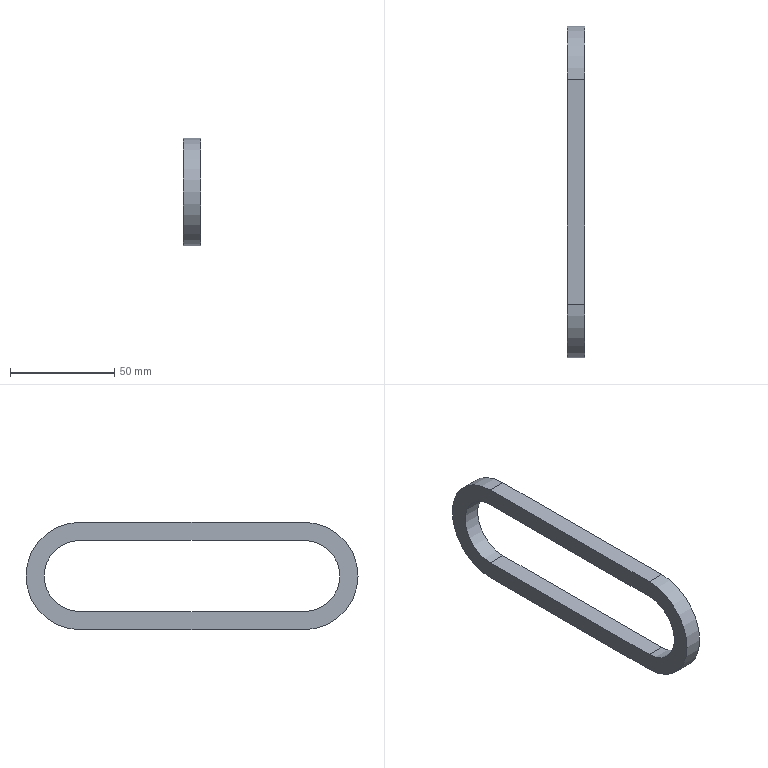Part | STEP file | 25B chain | 1 solid | 10 faces | box 8.6 x 159.55 x 51.6 mm | volume 26237 mm3 | plane 6 | cylinder 4 | commonest cylinder face diameters 34.2 x2 51.6 x2
STEP:
#1=CARTESIAN_POINT('',(0.,0.,0.));
#2=DIRECTION('',(0.,0.,1.));
#3=DIRECTION('',(1.,0.,0.));
#4=AXIS2_PLACEMENT_3D('',#1,#2,#3);
#5=CARTESIAN_POINT('',(8.6,107.95,-17.1));
#6=VERTEX_POINT('',#5);
#7=CARTESIAN_POINT('',(8.6,-0.000000004,-17.1));
#8=VERTEX_POINT('',#7);
#9=CARTESIAN_POINT('',(8.6,53.975,-17.1));
#10=DIRECTION('',(0.,-1.,0.));
#11=VECTOR('',#10,1.);
#12=LINE('',#9,#11);
#13=CARTESIAN_POINT('',(8.6,-26.757,25.8));
#14=DIRECTION('',(1.,0.,0.));
#15=DIRECTION('',(0.,0.,-1.));
#16=AXIS2_PLACEMENT_3D('',#13,#14,#15);
#17=PLANE('',#16);
#18=CARTESIAN_POINT('',(42.9,80.732));
#19=DIRECTION('',(0.,-1.));
#20=VECTOR('',#19,1.);
#21=LINE('',#18,#20);
#22=(GEOMETRIC_REPRESENTATION_CONTEXT(2)PARAMETRIC_REPRESENTATION_CONTEXT()REPRESENTATION_CONTEXT('',''));
#23=DEFINITIONAL_REPRESENTATION('',(#21),#22);
#24=PCURVE('',#17,#23);
#25=CARTESIAN_POINT('',(0.,107.95,-17.1));
#26=DIRECTION('',(0.,0.,1.));
#27=DIRECTION('',(0.,-1.,0.));
#28=AXIS2_PLACEMENT_3D('',#25,#26,#27);
#29=PLANE('',#28);
#30=CARTESIAN_POINT('',(53.975,8.6));
#31=DIRECTION('',(1.,0.));
#32=VECTOR('',#31,1.);
#33=LINE('',#30,#32);
#34=(GEOMETRIC_REPRESENTATION_CONTEXT(2)PARAMETRIC_REPRESENTATION_CONTEXT()REPRESENTATION_CONTEXT('',''));
#35=DEFINITIONAL_REPRESENTATION('',(#33),#34);
#36=PCURVE('',#29,#35);
#37=SURFACE_CURVE('',#12,(#24,#36),.PCURVE_S1.);
#38=EDGE_CURVE('',#6,#8,#37,.T.);
#39=ORIENTED_EDGE('',*,*,#38,.T.);
#40=CARTESIAN_POINT('',(8.6,-0.000000002,17.1));
#41=VERTEX_POINT('',#40);
#42=CARTESIAN_POINT('',(8.6,0.,0.));
#43=DIRECTION('',(-1.,0.,0.));
#44=DIRECTION('',(0.,0.,1.));
#45=AXIS2_PLACEMENT_3D('',#42,#43,#44);
#46=CIRCLE('',#45,17.1);
#47=CARTESIAN_POINT('',(8.7,26.757));
#48=CARTESIAN_POINT('',(8.7,56.375));
#49=CARTESIAN_POINT('',(34.35,41.566));
#50=CARTESIAN_POINT('',(60.,26.757));
#51=CARTESIAN_POINT('',(34.35,11.948));
#52=CARTESIAN_POINT('',(8.7,-2.861));
#53=CARTESIAN_POINT('',(8.7,26.757));
#54=(BOUNDED_CURVE()B_SPLINE_CURVE(2,(#47,#48,#49,#50,#51,#52,#53),.UNSPECIFIED.,.T.,.F.)B_SPLINE_CURVE_WITH_KNOTS((1,2,2,2,2,1),(-2.094,0.,2.094,4.189,6.283,8.378),.UNSPECIFIED.)CURVE()GEOMETRIC_REPRESENTATION_ITEM()RATIONAL_B_SPLINE_CURVE((1.,0.5,1.,0.5,1.,0.5,1.))REPRESENTATION_ITEM(''));
#55=(GEOMETRIC_REPRESENTATION_CONTEXT(2)PARAMETRIC_REPRESENTATION_CONTEXT()REPRESENTATION_CONTEXT('',''));
#56=DEFINITIONAL_REPRESENTATION('',(#54),#55);
#57=PCURVE('',#17,#56);
#58=CARTESIAN_POINT('',(8.6,0.,0.));
#59=DIRECTION('',(-1.,0.,0.));
#60=DIRECTION('',(0.,0.,1.));
#61=AXIS2_PLACEMENT_3D('',#58,#59,#60);
#62=CYLINDRICAL_SURFACE('',#61,17.1);
#63=CARTESIAN_POINT('',(0.,0.));
#64=DIRECTION('',(1.,0.));
#65=VECTOR('',#64,1.);
#66=LINE('',#63,#65);
#67=(GEOMETRIC_REPRESENTATION_CONTEXT(2)PARAMETRIC_REPRESENTATION_CONTEXT()REPRESENTATION_CONTEXT('',''));
#68=DEFINITIONAL_REPRESENTATION('',(#66),#67);
#69=PCURVE('',#62,#68);
#70=SURFACE_CURVE('',#46,(#57,#69),.PCURVE_S1.);
#71=EDGE_CURVE('',#8,#41,#70,.T.);
#72=ORIENTED_EDGE('',*,*,#71,.T.);
#73=CARTESIAN_POINT('',(8.6,107.95,17.1));
#74=VERTEX_POINT('',#73);
#75=CARTESIAN_POINT('',(8.6,53.975,17.1));
#76=DIRECTION('',(0.,1.,0.));
#77=VECTOR('',#76,1.);
#78=LINE('',#75,#77);
#79=CARTESIAN_POINT('',(8.7,80.732));
#80=DIRECTION('',(0.,1.));
#81=VECTOR('',#80,1.);
#82=LINE('',#79,#81);
#83=(GEOMETRIC_REPRESENTATION_CONTEXT(2)PARAMETRIC_REPRESENTATION_CONTEXT()REPRESENTATION_CONTEXT('',''));
#84=DEFINITIONAL_REPRESENTATION('',(#82),#83);
#85=PCURVE('',#17,#84);
#86=CARTESIAN_POINT('',(0.,0.,17.1));
#87=DIRECTION('',(0.,0.,-1.));
#88=DIRECTION('',(0.,1.,0.));
#89=AXIS2_PLACEMENT_3D('',#86,#87,#88);
#90=PLANE('',#89);
#91=CARTESIAN_POINT('',(53.975,8.6));
#92=DIRECTION('',(1.,0.));
#93=VECTOR('',#92,1.);
#94=LINE('',#91,#93);
#95=(GEOMETRIC_REPRESENTATION_CONTEXT(2)PARAMETRIC_REPRESENTATION_CONTEXT()REPRESENTATION_CONTEXT('',''));
#96=DEFINITIONAL_REPRESENTATION('',(#94),#95);
#97=PCURVE('',#90,#96);
#98=SURFACE_CURVE('',#78,(#85,#97),.PCURVE_S1.);
#99=EDGE_CURVE('',#41,#74,#98,.T.);
#100=ORIENTED_EDGE('',*,*,#99,.T.);
#101=CARTESIAN_POINT('',(8.6,107.95,0.));
#102=DIRECTION('',(-1.,0.,0.));
#103=DIRECTION('',(0.,0.,1.));
#104=AXIS2_PLACEMENT_3D('',#101,#102,#103);
#105=CIRCLE('',#104,17.1);
#106=CARTESIAN_POINT('',(8.7,134.707));
#107=CARTESIAN_POINT('',(8.7,164.325));
#108=CARTESIAN_POINT('',(34.35,149.516));
#109=CARTESIAN_POINT('',(60.,134.707));
#110=CARTESIAN_POINT('',(34.35,119.898));
#111=CARTESIAN_POINT('',(8.7,105.089));
#112=CARTESIAN_POINT('',(8.7,134.707));
#113=(BOUNDED_CURVE()B_SPLINE_CURVE(2,(#106,#107,#108,#109,#110,#111,#112),.UNSPECIFIED.,.T.,.F.)B_SPLINE_CURVE_WITH_KNOTS((1,2,2,2,2,1),(-2.094,0.,2.094,4.189,6.283,8.378),.UNSPECIFIED.)CURVE()GEOMETRIC_REPRESENTATION_ITEM()RATIONAL_B_SPLINE_CURVE((1.,0.5,1.,0.5,1.,0.5,1.))REPRESENTATION_ITEM(''));
#114=(GEOMETRIC_REPRESENTATION_CONTEXT(2)PARAMETRIC_REPRESENTATION_CONTEXT()REPRESENTATION_CONTEXT('',''));
#115=DEFINITIONAL_REPRESENTATION('',(#113),#114);
#116=PCURVE('',#17,#115);
#117=CARTESIAN_POINT('',(8.6,107.95,0.));
#118=DIRECTION('',(-1.,0.,0.));
#119=DIRECTION('',(0.,0.,1.));
#120=AXIS2_PLACEMENT_3D('',#117,#118,#119);
#121=CYLINDRICAL_SURFACE('',#120,17.1);
#122=CARTESIAN_POINT('',(0.,0.));
#123=DIRECTION('',(1.,0.));
#124=VECTOR('',#123,1.);
#125=LINE('',#122,#124);
#126=(GEOMETRIC_REPRESENTATION_CONTEXT(2)PARAMETRIC_REPRESENTATION_CONTEXT()REPRESENTATION_CONTEXT('',''));
#127=DEFINITIONAL_REPRESENTATION('',(#125),#126);
#128=PCURVE('',#121,#127);
#129=SURFACE_CURVE('',#105,(#116,#128),.PCURVE_S1.);
#130=EDGE_CURVE('',#74,#6,#129,.T.);
#131=ORIENTED_EDGE('',*,*,#130,.T.);
#132=EDGE_LOOP('',(#39,#72,#100,#131));
#133=FACE_BOUND('',#132,.T.);
#134=CARTESIAN_POINT('',(8.6,107.95,-25.8));
#135=VERTEX_POINT('',#134);
#136=CARTESIAN_POINT('',(8.6,107.95,25.8));
#137=VERTEX_POINT('',#136);
#138=CARTESIAN_POINT('',(8.6,107.95,0.));
#139=DIRECTION('',(1.,0.,0.));
#140=DIRECTION('',(0.,0.,1.));
#141=AXIS2_PLACEMENT_3D('',#138,#139,#140);
#142=CIRCLE('',#141,25.8);
#143=CARTESIAN_POINT('',(25.8,134.707));
#144=DIRECTION('',(-1.,0.));
#145=AXIS2_PLACEMENT_2D('',#143,#144);
#146=CIRCLE('',#145,25.8);
#147=(GEOMETRIC_REPRESENTATION_CONTEXT(2)PARAMETRIC_REPRESENTATION_CONTEXT()REPRESENTATION_CONTEXT('',''));
#148=DEFINITIONAL_REPRESENTATION('',(#146),#147);
#149=PCURVE('',#17,#148);
#150=CARTESIAN_POINT('',(8.6,107.95,0.));
#151=DIRECTION('',(-1.,0.,0.));
#152=DIRECTION('',(0.,0.,1.));
#153=AXIS2_PLACEMENT_3D('',#150,#151,#152);
#154=CYLINDRICAL_SURFACE('',#153,25.8);
#155=CARTESIAN_POINT('',(6.283,0.));
#156=DIRECTION('',(-1.,0.));
#157=VECTOR('',#156,1.);
#158=LINE('',#155,#157);
#159=(GEOMETRIC_REPRESENTATION_CONTEXT(2)PARAMETRIC_REPRESENTATION_CONTEXT()REPRESENTATION_CONTEXT('',''));
#160=DEFINITIONAL_REPRESENTATION('',(#158),#159);
#161=PCURVE('',#154,#160);
#162=SURFACE_CURVE('',#142,(#149,#161),.PCURVE_S1.);
#163=EDGE_CURVE('',#135,#137,#162,.T.);
#164=ORIENTED_EDGE('',*,*,#163,.T.);
#165=CARTESIAN_POINT('',(8.6,0.,25.8));
#166=VERTEX_POINT('',#165);
#167=CARTESIAN_POINT('',(8.6,53.975,25.8));
#168=DIRECTION('',(0.,-1.,0.));
#169=VECTOR('',#168,1.);
#170=LINE('',#167,#169);
#171=CARTESIAN_POINT('',(0.,80.732));
#172=DIRECTION('',(0.,-1.));
#173=VECTOR('',#172,1.);
#174=LINE('',#171,#173);
#175=(GEOMETRIC_REPRESENTATION_CONTEXT(2)PARAMETRIC_REPRESENTATION_CONTEXT()REPRESENTATION_CONTEXT('',''));
#176=DEFINITIONAL_REPRESENTATION('',(#174),#175);
#177=PCURVE('',#17,#176);
#178=CARTESIAN_POINT('',(8.6,0.,25.8));
#179=DIRECTION('',(0.,0.,-1.));
#180=DIRECTION('',(-1.,0.,0.));
#181=AXIS2_PLACEMENT_3D('',#178,#179,#180);
#182=PLANE('',#181);
#183=CARTESIAN_POINT('',(0.,53.975));
#184=DIRECTION('',(0.,-1.));
#185=VECTOR('',#184,1.);
#186=LINE('',#183,#185);
#187=(GEOMETRIC_REPRESENTATION_CONTEXT(2)PARAMETRIC_REPRESENTATION_CONTEXT()REPRESENTATION_CONTEXT('',''));
#188=DEFINITIONAL_REPRESENTATION('',(#186),#187);
#189=PCURVE('',#182,#188);
#190=SURFACE_CURVE('',#170,(#177,#189),.PCURVE_S1.);
#191=EDGE_CURVE('',#137,#166,#190,.T.);
#192=ORIENTED_EDGE('',*,*,#191,.T.);
#193=CARTESIAN_POINT('',(8.6,0.,-25.8));
#194=VERTEX_POINT('',#193);
#195=CARTESIAN_POINT('',(8.6,0.,0.));
#196=DIRECTION('',(1.,0.,0.));
#197=DIRECTION('',(0.,0.,1.));
#198=AXIS2_PLACEMENT_3D('',#195,#196,#197);
#199=CIRCLE('',#198,25.8);
#200=CARTESIAN_POINT('',(25.8,26.757));
#201=DIRECTION('',(-1.,0.));
#202=AXIS2_PLACEMENT_2D('',#200,#201);
#203=CIRCLE('',#202,25.8);
#204=(GEOMETRIC_REPRESENTATION_CONTEXT(2)PARAMETRIC_REPRESENTATION_CONTEXT()REPRESENTATION_CONTEXT('',''));
#205=DEFINITIONAL_REPRESENTATION('',(#203),#204);
#206=PCURVE('',#17,#205);
#207=CARTESIAN_POINT('',(8.6,0.,0.));
#208=DIRECTION('',(-1.,0.,0.));
#209=DIRECTION('',(0.,0.,1.));
#210=AXIS2_PLACEMENT_3D('',#207,#208,#209);
#211=CYLINDRICAL_SURFACE('',#210,25.8);
#212=CARTESIAN_POINT('',(6.283,0.));
#213=DIRECTION('',(-1.,0.));
#214=VECTOR('',#213,1.);
#215=LINE('',#212,#214);
#216=(GEOMETRIC_REPRESENTATION_CONTEXT(2)PARAMETRIC_REPRESENTATION_CONTEXT()REPRESENTATION_CONTEXT('',''));
#217=DEFINITIONAL_REPRESENTATION('',(#215),#216);
#218=PCURVE('',#211,#217);
#219=SURFACE_CURVE('',#199,(#206,#218),.PCURVE_S1.);
#220=EDGE_CURVE('',#166,#194,#219,.T.);
#221=ORIENTED_EDGE('',*,*,#220,.T.);
#222=CARTESIAN_POINT('',(8.6,53.975,-25.8));
#223=DIRECTION('',(0.,1.,0.));
#224=VECTOR('',#223,1.);
#225=LINE('',#222,#224);
#226=CARTESIAN_POINT('',(51.6,80.732));
#227=DIRECTION('',(0.,1.));
#228=VECTOR('',#227,1.);
#229=LINE('',#226,#228);
#230=(GEOMETRIC_REPRESENTATION_CONTEXT(2)PARAMETRIC_REPRESENTATION_CONTEXT()REPRESENTATION_CONTEXT('',''));
#231=DEFINITIONAL_REPRESENTATION('',(#229),#230);
#232=PCURVE('',#17,#231);
#233=CARTESIAN_POINT('',(0.,0.,-25.8));
#234=DIRECTION('',(0.,0.,1.));
#235=DIRECTION('',(1.,0.,0.));
#236=AXIS2_PLACEMENT_3D('',#233,#234,#235);
#237=PLANE('',#236);
#238=CARTESIAN_POINT('',(8.6,53.975));
#239=DIRECTION('',(0.,1.));
#240=VECTOR('',#239,1.);
#241=LINE('',#238,#240);
#242=(GEOMETRIC_REPRESENTATION_CONTEXT(2)PARAMETRIC_REPRESENTATION_CONTEXT()REPRESENTATION_CONTEXT('',''));
#243=DEFINITIONAL_REPRESENTATION('',(#241),#242);
#244=PCURVE('',#237,#243);
#245=SURFACE_CURVE('',#225,(#232,#244),.PCURVE_S1.);
#246=EDGE_CURVE('',#194,#135,#245,.T.);
#247=ORIENTED_EDGE('',*,*,#246,.T.);
#248=EDGE_LOOP('',(#164,#192,#221,#247));
#249=FACE_BOUND('',#248,.T.);
#250=ADVANCED_FACE('',(#133,#249),#17,.T.);
#251=CARTESIAN_POINT('',(0.,-0.000000002,17.1));
#252=VERTEX_POINT('',#251);
#253=CARTESIAN_POINT('',(4.3,-0.000000003,17.1));
#254=DIRECTION('',(1.,0.,0.));
#255=VECTOR('',#254,1.);
#256=LINE('',#253,#255);
#257=CARTESIAN_POINT('',(6.283,4.3));
#258=DIRECTION('',(0.,-1.));
#259=VECTOR('',#258,1.);
#260=LINE('',#257,#259);
#261=(GEOMETRIC_REPRESENTATION_CONTEXT(2)PARAMETRIC_REPRESENTATION_CONTEXT()REPRESENTATION_CONTEXT('',''));
#262=DEFINITIONAL_REPRESENTATION('',(#260),#261);
#263=PCURVE('',#62,#262);
#264=CARTESIAN_POINT('',(-0.000000003,4.3));
#265=DIRECTION('',(0.,1.));
#266=VECTOR('',#265,1.);
#267=LINE('',#264,#266);
#268=(GEOMETRIC_REPRESENTATION_CONTEXT(2)PARAMETRIC_REPRESENTATION_CONTEXT()REPRESENTATION_CONTEXT('',''));
#269=DEFINITIONAL_REPRESENTATION('',(#267),#268);
#270=PCURVE('',#90,#269);
#271=SURFACE_CURVE('',#256,(#263,#270),.PCURVE_S1.);
#272=EDGE_CURVE('',#252,#41,#271,.T.);
#273=ORIENTED_EDGE('',*,*,#272,.F.);
#274=CARTESIAN_POINT('',(0.,-0.000000004,-17.1));
#275=VERTEX_POINT('',#274);
#276=CARTESIAN_POINT('',(0.,0.,0.));
#277=DIRECTION('',(-1.,0.,0.));
#278=DIRECTION('',(0.,0.,1.));
#279=AXIS2_PLACEMENT_3D('',#276,#277,#278);
#280=CIRCLE('',#279,17.1);
#281=CARTESIAN_POINT('',(0.,8.6));
#282=DIRECTION('',(1.,0.));
#283=VECTOR('',#282,1.);
#284=LINE('',#281,#283);
#285=(GEOMETRIC_REPRESENTATION_CONTEXT(2)PARAMETRIC_REPRESENTATION_CONTEXT()REPRESENTATION_CONTEXT('',''));
#286=DEFINITIONAL_REPRESENTATION('',(#284),#285);
#287=PCURVE('',#62,#286);
#288=CARTESIAN_POINT('',(0.,-26.757,25.8));
#289=DIRECTION('',(1.,0.,0.));
#290=DIRECTION('',(0.,0.,-1.));
#291=AXIS2_PLACEMENT_3D('',#288,#289,#290);
#292=PLANE('',#291);
#293=CARTESIAN_POINT('',(8.7,26.757));
#294=CARTESIAN_POINT('',(8.7,56.375));
#295=CARTESIAN_POINT('',(34.35,41.566));
#296=CARTESIAN_POINT('',(60.,26.757));
#297=CARTESIAN_POINT('',(34.35,11.948));
#298=CARTESIAN_POINT('',(8.7,-2.861));
#299=CARTESIAN_POINT('',(8.7,26.757));
#300=(BOUNDED_CURVE()B_SPLINE_CURVE(2,(#293,#294,#295,#296,#297,#298,#299),.UNSPECIFIED.,.T.,.F.)B_SPLINE_CURVE_WITH_KNOTS((1,2,2,2,2,1),(-2.094,0.,2.094,4.189,6.283,8.378),.UNSPECIFIED.)CURVE()GEOMETRIC_REPRESENTATION_ITEM()RATIONAL_B_SPLINE_CURVE((1.,0.5,1.,0.5,1.,0.5,1.))REPRESENTATION_ITEM(''));
#301=(GEOMETRIC_REPRESENTATION_CONTEXT(2)PARAMETRIC_REPRESENTATION_CONTEXT()REPRESENTATION_CONTEXT('',''));
#302=DEFINITIONAL_REPRESENTATION('',(#300),#301);
#303=PCURVE('',#292,#302);
#304=SURFACE_CURVE('',#280,(#287,#303),.PCURVE_S1.);
#305=EDGE_CURVE('',#275,#252,#304,.T.);
#306=ORIENTED_EDGE('',*,*,#305,.F.);
#307=CARTESIAN_POINT('',(4.3,-0.000000007,-17.1));
#308=DIRECTION('',(-1.,0.,0.));
#309=VECTOR('',#308,1.);
#310=LINE('',#307,#309);
#311=CARTESIAN_POINT('',(3.142,4.3));
#312=DIRECTION('',(0.,1.));
#313=VECTOR('',#312,1.);
#314=LINE('',#311,#313);
#315=(GEOMETRIC_REPRESENTATION_CONTEXT(2)PARAMETRIC_REPRESENTATION_CONTEXT()REPRESENTATION_CONTEXT('',''));
#316=DEFINITIONAL_REPRESENTATION('',(#314),#315);
#317=PCURVE('',#62,#316);
#318=CARTESIAN_POINT('',(107.95,4.3));
#319=DIRECTION('',(0.,-1.));
#320=VECTOR('',#319,1.);
#321=LINE('',#318,#320);
#322=(GEOMETRIC_REPRESENTATION_CONTEXT(2)PARAMETRIC_REPRESENTATION_CONTEXT()REPRESENTATION_CONTEXT('',''));
#323=DEFINITIONAL_REPRESENTATION('',(#321),#322);
#324=PCURVE('',#29,#323);
#325=SURFACE_CURVE('',#310,(#317,#324),.PCURVE_S1.);
#326=EDGE_CURVE('',#8,#275,#325,.T.);
#327=ORIENTED_EDGE('',*,*,#326,.F.);
#328=ORIENTED_EDGE('',*,*,#71,.T.);
#329=EDGE_LOOP('',(#273,#306,#327,#328));
#330=FACE_BOUND('',#329,.F.);
#331=ADVANCED_FACE('',(#330),#62,.F.);
#332=ORIENTED_EDGE('',*,*,#38,.F.);
#333=CARTESIAN_POINT('',(0.,107.95,-17.1));
#334=VERTEX_POINT('',#333);
#335=CARTESIAN_POINT('',(4.3,107.95,-17.1));
#336=DIRECTION('',(-1.,0.,0.));
#337=VECTOR('',#336,1.);
#338=LINE('',#335,#337);
#339=CARTESIAN_POINT('',(0.,4.3));
#340=DIRECTION('',(0.,-1.));
#341=VECTOR('',#340,1.);
#342=LINE('',#339,#341);
#343=(GEOMETRIC_REPRESENTATION_CONTEXT(2)PARAMETRIC_REPRESENTATION_CONTEXT()REPRESENTATION_CONTEXT('',''));
#344=DEFINITIONAL_REPRESENTATION('',(#342),#343);
#345=PCURVE('',#29,#344);
#346=CARTESIAN_POINT('',(3.142,4.3));
#347=DIRECTION('',(0.,1.));
#348=VECTOR('',#347,1.);
#349=LINE('',#346,#348);
#350=(GEOMETRIC_REPRESENTATION_CONTEXT(2)PARAMETRIC_REPRESENTATION_CONTEXT()REPRESENTATION_CONTEXT('',''));
#351=DEFINITIONAL_REPRESENTATION('',(#349),#350);
#352=PCURVE('',#121,#351);
#353=SURFACE_CURVE('',#338,(#345,#352),.PCURVE_S1.);
#354=EDGE_CURVE('',#6,#334,#353,.T.);
#355=ORIENTED_EDGE('',*,*,#354,.T.);
#356=CARTESIAN_POINT('',(0.,53.975,-17.1));
#357=DIRECTION('',(0.,-1.,0.));
#358=VECTOR('',#357,1.);
#359=LINE('',#356,#358);
#360=CARTESIAN_POINT('',(53.975,0.));
#361=DIRECTION('',(1.,0.));
#362=VECTOR('',#361,1.);
#363=LINE('',#360,#362);
#364=(GEOMETRIC_REPRESENTATION_CONTEXT(2)PARAMETRIC_REPRESENTATION_CONTEXT()REPRESENTATION_CONTEXT('',''));
#365=DEFINITIONAL_REPRESENTATION('',(#363),#364);
#366=PCURVE('',#29,#365);
#367=CARTESIAN_POINT('',(42.9,80.732));
#368=DIRECTION('',(0.,-1.));
#369=VECTOR('',#368,1.);
#370=LINE('',#367,#369);
#371=(GEOMETRIC_REPRESENTATION_CONTEXT(2)PARAMETRIC_REPRESENTATION_CONTEXT()REPRESENTATION_CONTEXT('',''));
#372=DEFINITIONAL_REPRESENTATION('',(#370),#371);
#373=PCURVE('',#292,#372);
#374=SURFACE_CURVE('',#359,(#366,#373),.PCURVE_S1.);
#375=EDGE_CURVE('',#334,#275,#374,.T.);
#376=ORIENTED_EDGE('',*,*,#375,.T.);
#377=ORIENTED_EDGE('',*,*,#326,.F.);
#378=EDGE_LOOP('',(#332,#355,#376,#377));
#379=FACE_BOUND('',#378,.T.);
#380=ADVANCED_FACE('',(#379),#29,.T.);
#381=ORIENTED_EDGE('',*,*,#354,.T.);
#382=CARTESIAN_POINT('',(0.,107.95,17.1));
#383=VERTEX_POINT('',#382);
#384=CARTESIAN_POINT('',(0.,107.95,0.));
#385=DIRECTION('',(-1.,0.,0.));
#386=DIRECTION('',(0.,0.,1.));
#387=AXIS2_PLACEMENT_3D('',#384,#385,#386);
#388=CIRCLE('',#387,17.1);
#389=CARTESIAN_POINT('',(0.,8.6));
#390=DIRECTION('',(1.,0.));
#391=VECTOR('',#390,1.);
#392=LINE('',#389,#391);
#393=(GEOMETRIC_REPRESENTATION_CONTEXT(2)PARAMETRIC_REPRESENTATION_CONTEXT()REPRESENTATION_CONTEXT('',''));
#394=DEFINITIONAL_REPRESENTATION('',(#392),#393);
#395=PCURVE('',#121,#394);
#396=CARTESIAN_POINT('',(8.7,134.707));
#397=CARTESIAN_POINT('',(8.7,164.325));
#398=CARTESIAN_POINT('',(34.35,149.516));
#399=CARTESIAN_POINT('',(60.,134.707));
#400=CARTESIAN_POINT('',(34.35,119.898));
#401=CARTESIAN_POINT('',(8.7,105.089));
#402=CARTESIAN_POINT('',(8.7,134.707));
#403=(BOUNDED_CURVE()B_SPLINE_CURVE(2,(#396,#397,#398,#399,#400,#401,#402),.UNSPECIFIED.,.T.,.F.)B_SPLINE_CURVE_WITH_KNOTS((1,2,2,2,2,1),(-2.094,0.,2.094,4.189,6.283,8.378),.UNSPECIFIED.)CURVE()GEOMETRIC_REPRESENTATION_ITEM()RATIONAL_B_SPLINE_CURVE((1.,0.5,1.,0.5,1.,0.5,1.))REPRESENTATION_ITEM(''));
#404=(GEOMETRIC_REPRESENTATION_CONTEXT(2)PARAMETRIC_REPRESENTATION_CONTEXT()REPRESENTATION_CONTEXT('',''));
#405=DEFINITIONAL_REPRESENTATION('',(#403),#404);
#406=PCURVE('',#292,#405);
#407=SURFACE_CURVE('',#388,(#395,#406),.PCURVE_S1.);
#408=EDGE_CURVE('',#383,#334,#407,.T.);
#409=ORIENTED_EDGE('',*,*,#408,.F.);
#410=CARTESIAN_POINT('',(4.3,107.95,17.1));
#411=DIRECTION('',(-1.,0.,0.));
#412=VECTOR('',#411,1.);
#413=LINE('',#410,#412);
#414=CARTESIAN_POINT('',(0.,4.3));
#415=DIRECTION('',(0.,1.));
#416=VECTOR('',#415,1.);
#417=LINE('',#414,#416);
#418=(GEOMETRIC_REPRESENTATION_CONTEXT(2)PARAMETRIC_REPRESENTATION_CONTEXT()REPRESENTATION_CONTEXT('',''));
#419=DEFINITIONAL_REPRESENTATION('',(#417),#418);
#420=PCURVE('',#121,#419);
#421=CARTESIAN_POINT('',(107.95,4.3));
#422=DIRECTION('',(0.,-1.));
#423=VECTOR('',#422,1.);
#424=LINE('',#421,#423);
#425=(GEOMETRIC_REPRESENTATION_CONTEXT(2)PARAMETRIC_REPRESENTATION_CONTEXT()REPRESENTATION_CONTEXT('',''));
#426=DEFINITIONAL_REPRESENTATION('',(#424),#425);
#427=PCURVE('',#90,#426);
#428=SURFACE_CURVE('',#413,(#420,#427),.PCURVE_S1.);
#429=EDGE_CURVE('',#74,#383,#428,.T.);
#430=ORIENTED_EDGE('',*,*,#429,.F.);
#431=ORIENTED_EDGE('',*,*,#130,.T.);
#432=EDGE_LOOP('',(#381,#409,#430,#431));
#433=FACE_BOUND('',#432,.F.);
#434=ADVANCED_FACE('',(#433),#121,.F.);
#435=ORIENTED_EDGE('',*,*,#99,.F.);
#436=ORIENTED_EDGE('',*,*,#272,.F.);
#437=CARTESIAN_POINT('',(0.,53.975,17.1));
#438=DIRECTION('',(0.,1.,0.));
#439=VECTOR('',#438,1.);
#440=LINE('',#437,#439);
#441=CARTESIAN_POINT('',(53.975,0.));
#442=DIRECTION('',(1.,0.));
#443=VECTOR('',#442,1.);
#444=LINE('',#441,#443);
#445=(GEOMETRIC_REPRESENTATION_CONTEXT(2)PARAMETRIC_REPRESENTATION_CONTEXT()REPRESENTATION_CONTEXT('',''));
#446=DEFINITIONAL_REPRESENTATION('',(#444),#445);
#447=PCURVE('',#90,#446);
#448=CARTESIAN_POINT('',(8.7,80.732));
#449=DIRECTION('',(0.,1.));
#450=VECTOR('',#449,1.);
#451=LINE('',#448,#450);
#452=(GEOMETRIC_REPRESENTATION_CONTEXT(2)PARAMETRIC_REPRESENTATION_CONTEXT()REPRESENTATION_CONTEXT('',''));
#453=DEFINITIONAL_REPRESENTATION('',(#451),#452);
#454=PCURVE('',#292,#453);
#455=SURFACE_CURVE('',#440,(#447,#454),.PCURVE_S1.);
#456=EDGE_CURVE('',#252,#383,#455,.T.);
#457=ORIENTED_EDGE('',*,*,#456,.T.);
#458=ORIENTED_EDGE('',*,*,#429,.F.);
#459=EDGE_LOOP('',(#435,#436,#457,#458));
#460=FACE_BOUND('',#459,.T.);
#461=ADVANCED_FACE('',(#460),#90,.T.);
#462=CARTESIAN_POINT('',(0.,0.,25.8));
#463=VERTEX_POINT('',#462);
#464=CARTESIAN_POINT('',(4.3,0.,25.8));
#465=DIRECTION('',(-1.,0.,0.));
#466=VECTOR('',#465,1.);
#467=LINE('',#464,#466);
#468=CARTESIAN_POINT('',(4.3,0.));
#469=DIRECTION('',(1.,0.));
#470=VECTOR('',#469,1.);
#471=LINE('',#468,#470);
#472=(GEOMETRIC_REPRESENTATION_CONTEXT(2)PARAMETRIC_REPRESENTATION_CONTEXT()REPRESENTATION_CONTEXT('',''));
#473=DEFINITIONAL_REPRESENTATION('',(#471),#472);
#474=PCURVE('',#182,#473);
#475=CARTESIAN_POINT('',(6.283,4.3));
#476=DIRECTION('',(0.,1.));
#477=VECTOR('',#476,1.);
#478=LINE('',#475,#477);
#479=(GEOMETRIC_REPRESENTATION_CONTEXT(2)PARAMETRIC_REPRESENTATION_CONTEXT()REPRESENTATION_CONTEXT('',''));
#480=DEFINITIONAL_REPRESENTATION('',(#478),#479);
#481=PCURVE('',#211,#480);
#482=SURFACE_CURVE('',#467,(#474,#481),.PCURVE_S1.);
#483=EDGE_CURVE('',#166,#463,#482,.T.);
#484=ORIENTED_EDGE('',*,*,#483,.F.);
#485=ORIENTED_EDGE('',*,*,#191,.F.);
#486=CARTESIAN_POINT('',(0.,107.95,25.8));
#487=VERTEX_POINT('',#486);
#488=CARTESIAN_POINT('',(4.3,107.95,25.8));
#489=DIRECTION('',(1.,0.,0.));
#490=VECTOR('',#489,1.);
#491=LINE('',#488,#490);
#492=CARTESIAN_POINT('',(4.3,107.95));
#493=DIRECTION('',(-1.,0.));
#494=VECTOR('',#493,1.);
#495=LINE('',#492,#494);
#496=(GEOMETRIC_REPRESENTATION_CONTEXT(2)PARAMETRIC_REPRESENTATION_CONTEXT()REPRESENTATION_CONTEXT('',''));
#497=DEFINITIONAL_REPRESENTATION('',(#495),#496);
#498=PCURVE('',#182,#497);
#499=CARTESIAN_POINT('',(0.,4.3));
#500=DIRECTION('',(0.,-1.));
#501=VECTOR('',#500,1.);
#502=LINE('',#499,#501);
#503=(GEOMETRIC_REPRESENTATION_CONTEXT(2)PARAMETRIC_REPRESENTATION_CONTEXT()REPRESENTATION_CONTEXT('',''));
#504=DEFINITIONAL_REPRESENTATION('',(#502),#503);
#505=PCURVE('',#154,#504);
#506=SURFACE_CURVE('',#491,(#498,#505),.PCURVE_S1.);
#507=EDGE_CURVE('',#487,#137,#506,.T.);
#508=ORIENTED_EDGE('',*,*,#507,.F.);
#509=CARTESIAN_POINT('',(0.,53.975,25.8));
#510=DIRECTION('',(0.,1.,0.));
#511=VECTOR('',#510,1.);
#512=LINE('',#509,#511);
#513=CARTESIAN_POINT('',(8.6,53.975));
#514=DIRECTION('',(0.,1.));
#515=VECTOR('',#514,1.);
#516=LINE('',#513,#515);
#517=(GEOMETRIC_REPRESENTATION_CONTEXT(2)PARAMETRIC_REPRESENTATION_CONTEXT()REPRESENTATION_CONTEXT('',''));
#518=DEFINITIONAL_REPRESENTATION('',(#516),#517);
#519=PCURVE('',#182,#518);
#520=CARTESIAN_POINT('',(0.,80.732));
#521=DIRECTION('',(0.,1.));
#522=VECTOR('',#521,1.);
#523=LINE('',#520,#522);
#524=(GEOMETRIC_REPRESENTATION_CONTEXT(2)PARAMETRIC_REPRESENTATION_CONTEXT()REPRESENTATION_CONTEXT('',''));
#525=DEFINITIONAL_REPRESENTATION('',(#523),#524);
#526=PCURVE('',#292,#525);
#527=SURFACE_CURVE('',#512,(#519,#526),.PCURVE_S1.);
#528=EDGE_CURVE('',#463,#487,#527,.T.);
#529=ORIENTED_EDGE('',*,*,#528,.F.);
#530=EDGE_LOOP('',(#484,#485,#508,#529));
#531=FACE_BOUND('',#530,.T.);
#532=ADVANCED_FACE('',(#531),#182,.F.);
#533=ORIENTED_EDGE('',*,*,#507,.T.);
#534=ORIENTED_EDGE('',*,*,#163,.F.);
#535=CARTESIAN_POINT('',(0.,107.95,-25.8));
#536=VERTEX_POINT('',#535);
#537=CARTESIAN_POINT('',(4.3,107.95,-25.8));
#538=DIRECTION('',(1.,0.,0.));
#539=VECTOR('',#538,1.);
#540=LINE('',#537,#539);
#541=CARTESIAN_POINT('',(3.142,4.3));
#542=DIRECTION('',(0.,-1.));
#543=VECTOR('',#542,1.);
#544=LINE('',#541,#543);
#545=(GEOMETRIC_REPRESENTATION_CONTEXT(2)PARAMETRIC_REPRESENTATION_CONTEXT()REPRESENTATION_CONTEXT('',''));
#546=DEFINITIONAL_REPRESENTATION('',(#544),#545);
#547=PCURVE('',#154,#546);
#548=CARTESIAN_POINT('',(4.3,107.95));
#549=DIRECTION('',(1.,0.));
#550=VECTOR('',#549,1.);
#551=LINE('',#548,#550);
#552=(GEOMETRIC_REPRESENTATION_CONTEXT(2)PARAMETRIC_REPRESENTATION_CONTEXT()REPRESENTATION_CONTEXT('',''));
#553=DEFINITIONAL_REPRESENTATION('',(#551),#552);
#554=PCURVE('',#237,#553);
#555=SURFACE_CURVE('',#540,(#547,#554),.PCURVE_S1.);
#556=EDGE_CURVE('',#536,#135,#555,.T.);
#557=ORIENTED_EDGE('',*,*,#556,.F.);
#558=CARTESIAN_POINT('',(0.,107.95,0.));
#559=DIRECTION('',(-1.,0.,0.));
#560=DIRECTION('',(0.,0.,1.));
#561=AXIS2_PLACEMENT_3D('',#558,#559,#560);
#562=CIRCLE('',#561,25.8);
#563=CARTESIAN_POINT('',(0.,8.6));
#564=DIRECTION('',(1.,0.));
#565=VECTOR('',#564,1.);
#566=LINE('',#563,#565);
#567=(GEOMETRIC_REPRESENTATION_CONTEXT(2)PARAMETRIC_REPRESENTATION_CONTEXT()REPRESENTATION_CONTEXT('',''));
#568=DEFINITIONAL_REPRESENTATION('',(#566),#567);
#569=PCURVE('',#154,#568);
#570=CARTESIAN_POINT('',(0.,134.707));
#571=CARTESIAN_POINT('',(0.,179.394));
#572=CARTESIAN_POINT('',(38.7,157.051));
#573=CARTESIAN_POINT('',(77.4,134.707));
#574=CARTESIAN_POINT('',(38.7,112.364));
#575=CARTESIAN_POINT('',(0.,90.02));
#576=CARTESIAN_POINT('',(0.,134.707));
#577=(BOUNDED_CURVE()B_SPLINE_CURVE(2,(#570,#571,#572,#573,#574,#575,#576),.UNSPECIFIED.,.T.,.F.)B_SPLINE_CURVE_WITH_KNOTS((1,2,2,2,2,1),(-2.094,0.,2.094,4.189,6.283,8.378),.UNSPECIFIED.)CURVE()GEOMETRIC_REPRESENTATION_ITEM()RATIONAL_B_SPLINE_CURVE((1.,0.5,1.,0.5,1.,0.5,1.))REPRESENTATION_ITEM(''));
#578=(GEOMETRIC_REPRESENTATION_CONTEXT(2)PARAMETRIC_REPRESENTATION_CONTEXT()REPRESENTATION_CONTEXT('',''));
#579=DEFINITIONAL_REPRESENTATION('',(#577),#578);
#580=PCURVE('',#292,#579);
#581=SURFACE_CURVE('',#562,(#569,#580),.PCURVE_S1.);
#582=EDGE_CURVE('',#487,#536,#581,.T.);
#583=ORIENTED_EDGE('',*,*,#582,.F.);
#584=EDGE_LOOP('',(#533,#534,#557,#583));
#585=FACE_BOUND('',#584,.T.);
#586=ADVANCED_FACE('',(#585),#154,.T.);
#587=ORIENTED_EDGE('',*,*,#556,.T.);
#588=ORIENTED_EDGE('',*,*,#246,.F.);
#589=CARTESIAN_POINT('',(0.,0.,-25.8));
#590=VERTEX_POINT('',#589);
#591=CARTESIAN_POINT('',(4.3,0.,-25.8));
#592=DIRECTION('',(1.,0.,0.));
#593=VECTOR('',#592,1.);
#594=LINE('',#591,#593);
#595=CARTESIAN_POINT('',(4.3,0.));
#596=DIRECTION('',(1.,0.));
#597=VECTOR('',#596,1.);
#598=LINE('',#595,#597);
#599=(GEOMETRIC_REPRESENTATION_CONTEXT(2)PARAMETRIC_REPRESENTATION_CONTEXT()REPRESENTATION_CONTEXT('',''));
#600=DEFINITIONAL_REPRESENTATION('',(#598),#599);
#601=PCURVE('',#237,#600);
#602=CARTESIAN_POINT('',(3.142,4.3));
#603=DIRECTION('',(0.,-1.));
#604=VECTOR('',#603,1.);
#605=LINE('',#602,#604);
#606=(GEOMETRIC_REPRESENTATION_CONTEXT(2)PARAMETRIC_REPRESENTATION_CONTEXT()REPRESENTATION_CONTEXT('',''));
#607=DEFINITIONAL_REPRESENTATION('',(#605),#606);
#608=PCURVE('',#211,#607);
#609=SURFACE_CURVE('',#594,(#601,#608),.PCURVE_S1.);
#610=EDGE_CURVE('',#590,#194,#609,.T.);
#611=ORIENTED_EDGE('',*,*,#610,.F.);
#612=CARTESIAN_POINT('',(0.,53.975,-25.8));
#613=DIRECTION('',(0.,-1.,0.));
#614=VECTOR('',#613,1.);
#615=LINE('',#612,#614);
#616=CARTESIAN_POINT('',(0.,53.975));
#617=DIRECTION('',(0.,-1.));
#618=VECTOR('',#617,1.);
#619=LINE('',#616,#618);
#620=(GEOMETRIC_REPRESENTATION_CONTEXT(2)PARAMETRIC_REPRESENTATION_CONTEXT()REPRESENTATION_CONTEXT('',''));
#621=DEFINITIONAL_REPRESENTATION('',(#619),#620);
#622=PCURVE('',#237,#621);
#623=CARTESIAN_POINT('',(51.6,80.732));
#624=DIRECTION('',(0.,-1.));
#625=VECTOR('',#624,1.);
#626=LINE('',#623,#625);
#627=(GEOMETRIC_REPRESENTATION_CONTEXT(2)PARAMETRIC_REPRESENTATION_CONTEXT()REPRESENTATION_CONTEXT('',''));
#628=DEFINITIONAL_REPRESENTATION('',(#626),#627);
#629=PCURVE('',#292,#628);
#630=SURFACE_CURVE('',#615,(#622,#629),.PCURVE_S1.);
#631=EDGE_CURVE('',#536,#590,#630,.T.);
#632=ORIENTED_EDGE('',*,*,#631,.F.);
#633=EDGE_LOOP('',(#587,#588,#611,#632));
#634=FACE_BOUND('',#633,.T.);
#635=ADVANCED_FACE('',(#634),#237,.F.);
#636=ORIENTED_EDGE('',*,*,#610,.T.);
#637=ORIENTED_EDGE('',*,*,#220,.F.);
#638=ORIENTED_EDGE('',*,*,#483,.T.);
#639=CARTESIAN_POINT('',(0.,0.,0.));
#640=DIRECTION('',(-1.,0.,0.));
#641=DIRECTION('',(0.,0.,1.));
#642=AXIS2_PLACEMENT_3D('',#639,#640,#641);
#643=CIRCLE('',#642,25.8);
#644=CARTESIAN_POINT('',(0.,8.6));
#645=DIRECTION('',(1.,0.));
#646=VECTOR('',#645,1.);
#647=LINE('',#644,#646);
#648=(GEOMETRIC_REPRESENTATION_CONTEXT(2)PARAMETRIC_REPRESENTATION_CONTEXT()REPRESENTATION_CONTEXT('',''));
#649=DEFINITIONAL_REPRESENTATION('',(#647),#648);
#650=PCURVE('',#211,#649);
#651=CARTESIAN_POINT('',(0.,26.757));
#652=CARTESIAN_POINT('',(0.,71.444));
#653=CARTESIAN_POINT('',(38.7,49.101));
#654=CARTESIAN_POINT('',(77.4,26.757));
#655=CARTESIAN_POINT('',(38.7,4.414));
#656=CARTESIAN_POINT('',(0.,-17.93));
#657=CARTESIAN_POINT('',(0.,26.757));
#658=(BOUNDED_CURVE()B_SPLINE_CURVE(2,(#651,#652,#653,#654,#655,#656,#657),.UNSPECIFIED.,.T.,.F.)B_SPLINE_CURVE_WITH_KNOTS((1,2,2,2,2,1),(-2.094,0.,2.094,4.189,6.283,8.378),.UNSPECIFIED.)CURVE()GEOMETRIC_REPRESENTATION_ITEM()RATIONAL_B_SPLINE_CURVE((1.,0.5,1.,0.5,1.,0.5,1.))REPRESENTATION_ITEM(''));
#659=(GEOMETRIC_REPRESENTATION_CONTEXT(2)PARAMETRIC_REPRESENTATION_CONTEXT()REPRESENTATION_CONTEXT('',''));
#660=DEFINITIONAL_REPRESENTATION('',(#658),#659);
#661=PCURVE('',#292,#660);
#662=SURFACE_CURVE('',#643,(#650,#661),.PCURVE_S1.);
#663=EDGE_CURVE('',#590,#463,#662,.T.);
#664=ORIENTED_EDGE('',*,*,#663,.F.);
#665=EDGE_LOOP('',(#636,#637,#638,#664));
#666=FACE_BOUND('',#665,.T.);
#667=ADVANCED_FACE('',(#666),#211,.T.);
#668=ORIENTED_EDGE('',*,*,#456,.F.);
#669=ORIENTED_EDGE('',*,*,#305,.F.);
#670=ORIENTED_EDGE('',*,*,#375,.F.);
#671=ORIENTED_EDGE('',*,*,#408,.F.);
#672=EDGE_LOOP('',(#668,#669,#670,#671));
#673=FACE_BOUND('',#672,.T.);
#674=ORIENTED_EDGE('',*,*,#528,.T.);
#675=ORIENTED_EDGE('',*,*,#582,.T.);
#676=ORIENTED_EDGE('',*,*,#631,.T.);
#677=ORIENTED_EDGE('',*,*,#663,.T.);
#678=EDGE_LOOP('',(#674,#675,#676,#677));
#679=FACE_BOUND('',#678,.T.);
#680=ADVANCED_FACE('',(#673,#679),#292,.F.);
#681=CLOSED_SHELL('',(#250,#331,#380,#434,#461,#532,#586,#635,#667,#680));
#682=MANIFOLD_SOLID_BREP('',#681);
#683=(LENGTH_UNIT()NAMED_UNIT(*)SI_UNIT(.MILLI.,.METRE.));
#684=UNCERTAINTY_MEASURE_WITH_UNIT(LENGTH_MEASURE(0.0000001),#683,'','');
#685=(NAMED_UNIT(*)PLANE_ANGLE_UNIT()SI_UNIT($,.RADIAN.));
#686=(NAMED_UNIT(*)SI_UNIT($,.STERADIAN.)SOLID_ANGLE_UNIT());
#687=(GEOMETRIC_REPRESENTATION_CONTEXT(3)GLOBAL_UNCERTAINTY_ASSIGNED_CONTEXT((#684))GLOBAL_UNIT_ASSIGNED_CONTEXT((#683,#685,#686))REPRESENTATION_CONTEXT('',''));
#688=ADVANCED_BREP_SHAPE_REPRESENTATION('',(#4,#682),#687);